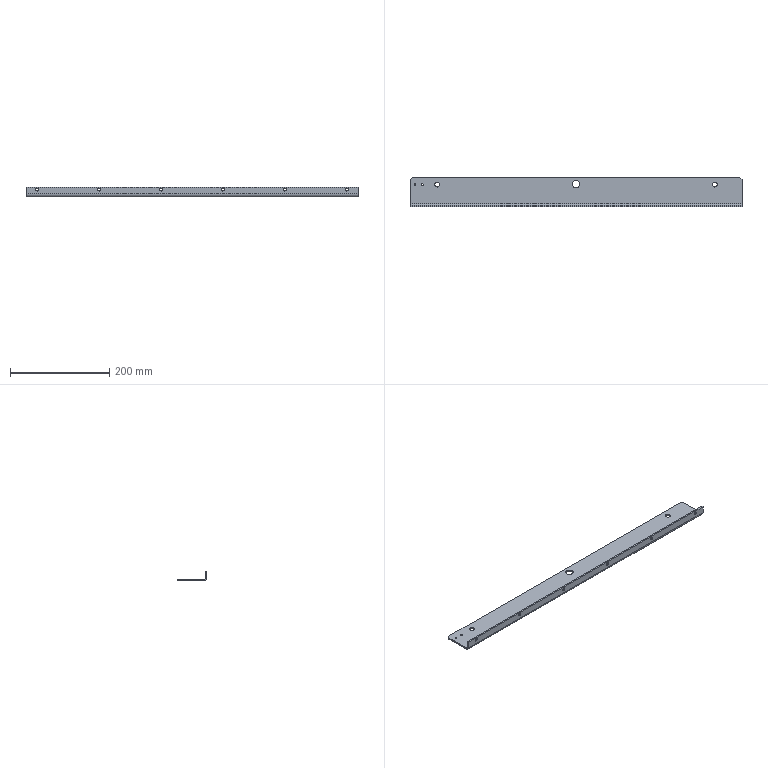Part | NX | features solid 2 | 1 solid | 34 faces | box 670 x 60 x 20 mm | volume 149246 mm3 | cylinder 24 | plane 10 | commonest cylinder face diameters 6 x13 3.459 x4 10 x4 15 x2 12 x1
STEP:
#1=CARTESIAN_POINT('',(-248.27,-1514.473,1300.));
#2=VERTEX_POINT('',#1);
#3=CARTESIAN_POINT('',(-248.27,-1514.473,1303.));
#4=VERTEX_POINT('',#3);
#5=CARTESIAN_POINT('',(-248.27,-1514.473,630.022));
#6=DIRECTION('',(0.,0.,1.));
#7=VECTOR('',#6,1000.);
#8=LINE('',#5,#7);
#9=EDGE_CURVE('',#2,#4,#8,.T.);
#10=ORIENTED_EDGE('',*,*,#9,.F.);
#11=CARTESIAN_POINT('',(-251.73,-1514.473,1300.));
#12=VERTEX_POINT('',#11);
#13=CARTESIAN_POINT('',(-250.,-1514.473,1300.));
#14=DIRECTION('',(0.,0.,-1.));
#15=DIRECTION('',(1.,0.,0.));
#16=AXIS2_PLACEMENT_3D('',#13,#14,#15);
#17=CIRCLE('',#16,1.73);
#18=EDGE_CURVE('',#2,#12,#17,.T.);
#19=ORIENTED_EDGE('',*,*,#18,.T.);
#20=CARTESIAN_POINT('',(-251.73,-1514.473,1303.));
#21=VERTEX_POINT('',#20);
#22=CARTESIAN_POINT('',(-251.73,-1514.473,630.022));
#23=DIRECTION('',(0.,0.,1.));
#24=VECTOR('',#23,1000.);
#25=LINE('',#22,#24);
#26=EDGE_CURVE('',#21,#12,#25,.F.);
#27=ORIENTED_EDGE('',*,*,#26,.F.);
#28=CARTESIAN_POINT('',(-250.,-1514.473,1303.));
#29=DIRECTION('',(0.,0.,1.));
#30=DIRECTION('',(-1.,0.,0.));
#31=AXIS2_PLACEMENT_3D('',#28,#29,#30);
#32=CIRCLE('',#31,1.73);
#33=EDGE_CURVE('',#21,#4,#32,.T.);
#34=ORIENTED_EDGE('',*,*,#33,.T.);
#35=EDGE_LOOP('',(#10,#19,#27,#34));
#36=FACE_BOUND('',#35,.T.);
#37=CARTESIAN_POINT('',(-250.,-1514.473,630.022));
#38=DIRECTION('',(0.,0.,1.));
#39=DIRECTION('',(-1.,0.,0.));
#40=AXIS2_PLACEMENT_3D('',#37,#38,#39);
#41=CYLINDRICAL_SURFACE('',#40,1.73);
#42=ADVANCED_FACE('',(#36),#41,.F.);
#43=CARTESIAN_POINT('',(-233.27,-1514.473,1303.));
#44=VERTEX_POINT('',#43);
#45=CARTESIAN_POINT('',(-233.27,-1514.473,1300.));
#46=VERTEX_POINT('',#45);
#47=CARTESIAN_POINT('',(-233.27,-1514.473,630.022));
#48=DIRECTION('',(0.,0.,1.));
#49=VECTOR('',#48,1000.);
#50=LINE('',#47,#49);
#51=EDGE_CURVE('',#44,#46,#50,.F.);
#52=ORIENTED_EDGE('',*,*,#51,.T.);
#53=CARTESIAN_POINT('',(-236.73,-1514.473,1300.));
#54=VERTEX_POINT('',#53);
#55=CARTESIAN_POINT('',(-235.,-1514.473,1300.));
#56=DIRECTION('',(0.,0.,-1.));
#57=DIRECTION('',(1.,0.,0.));
#58=AXIS2_PLACEMENT_3D('',#55,#56,#57);
#59=CIRCLE('',#58,1.73);
#60=EDGE_CURVE('',#46,#54,#59,.T.);
#61=ORIENTED_EDGE('',*,*,#60,.T.);
#62=CARTESIAN_POINT('',(-236.73,-1514.473,1303.));
#63=VERTEX_POINT('',#62);
#64=CARTESIAN_POINT('',(-236.73,-1514.473,630.022));
#65=DIRECTION('',(0.,0.,1.));
#66=VECTOR('',#65,1000.);
#67=LINE('',#64,#66);
#68=EDGE_CURVE('',#54,#63,#67,.T.);
#69=ORIENTED_EDGE('',*,*,#68,.T.);
#70=CARTESIAN_POINT('',(-235.,-1514.473,1303.));
#71=DIRECTION('',(0.,0.,1.));
#72=DIRECTION('',(-1.,0.,0.));
#73=AXIS2_PLACEMENT_3D('',#70,#71,#72);
#74=CIRCLE('',#73,1.73);
#75=EDGE_CURVE('',#63,#44,#74,.T.);
#76=ORIENTED_EDGE('',*,*,#75,.T.);
#77=EDGE_LOOP('',(#52,#61,#69,#76));
#78=FACE_BOUND('',#77,.T.);
#79=CARTESIAN_POINT('',(-235.,-1514.473,630.022));
#80=DIRECTION('',(0.,0.,1.));
#81=DIRECTION('',(-1.,0.,0.));
#82=AXIS2_PLACEMENT_3D('',#79,#80,#81);
#83=CYLINDRICAL_SURFACE('',#82,1.73);
#84=ADVANCED_FACE('',(#78),#83,.F.);
#85=CARTESIAN_POINT('',(82.5,-1513.723,1300.));
#86=VERTEX_POINT('',#85);
#87=CARTESIAN_POINT('',(82.5,-1513.723,1303.));
#88=VERTEX_POINT('',#87);
#89=CARTESIAN_POINT('',(82.5,-1513.723,630.022));
#90=DIRECTION('',(0.,0.,1.));
#91=VECTOR('',#90,1000.);
#92=LINE('',#89,#91);
#93=EDGE_CURVE('',#86,#88,#92,.T.);
#94=ORIENTED_EDGE('',*,*,#93,.F.);
#95=CARTESIAN_POINT('',(67.5,-1513.723,1300.));
#96=VERTEX_POINT('',#95);
#97=CARTESIAN_POINT('',(75.,-1513.723,1300.));
#98=DIRECTION('',(0.,0.,-1.));
#99=DIRECTION('',(1.,0.,0.));
#100=AXIS2_PLACEMENT_3D('',#97,#98,#99);
#101=CIRCLE('',#100,7.5);
#102=EDGE_CURVE('',#86,#96,#101,.T.);
#103=ORIENTED_EDGE('',*,*,#102,.T.);
#104=CARTESIAN_POINT('',(67.5,-1513.723,1303.));
#105=VERTEX_POINT('',#104);
#106=CARTESIAN_POINT('',(67.5,-1513.723,630.022));
#107=DIRECTION('',(0.,0.,1.));
#108=VECTOR('',#107,1000.);
#109=LINE('',#106,#108);
#110=EDGE_CURVE('',#105,#96,#109,.F.);
#111=ORIENTED_EDGE('',*,*,#110,.F.);
#112=CARTESIAN_POINT('',(75.,-1513.723,1303.));
#113=DIRECTION('',(0.,0.,1.));
#114=DIRECTION('',(1.,0.,0.));
#115=AXIS2_PLACEMENT_3D('',#112,#113,#114);
#116=CIRCLE('',#115,7.5);
#117=EDGE_CURVE('',#105,#88,#116,.T.);
#118=ORIENTED_EDGE('',*,*,#117,.T.);
#119=EDGE_LOOP('',(#94,#103,#111,#118));
#120=FACE_BOUND('',#119,.T.);
#121=CARTESIAN_POINT('',(75.,-1513.723,630.022));
#122=DIRECTION('',(0.,0.,1.));
#123=DIRECTION('',(-1.,0.,0.));
#124=AXIS2_PLACEMENT_3D('',#121,#122,#123);
#125=CYLINDRICAL_SURFACE('',#124,7.5);
#126=ADVANCED_FACE('',(#120),#125,.F.);
#127=CARTESIAN_POINT('',(-255.,-1499.473,1303.));
#128=VERTEX_POINT('',#127);
#129=CARTESIAN_POINT('',(-260.,-1504.473,1303.));
#130=VERTEX_POINT('',#129);
#131=CARTESIAN_POINT('',(-260.,-1504.473,1303.));
#132=DIRECTION('',(-0.7071,-0.7071,0.));
#133=VECTOR('',#132,1000.);
#134=LINE('',#131,#133);
#135=EDGE_CURVE('',#128,#130,#134,.T.);
#136=ORIENTED_EDGE('',*,*,#135,.F.);
#137=CARTESIAN_POINT('',(-255.,-1499.473,1300.));
#138=VERTEX_POINT('',#137);
#139=CARTESIAN_POINT('',(-255.,-1499.473,1300.));
#140=DIRECTION('',(0.,0.,1.));
#141=VECTOR('',#140,1000.);
#142=LINE('',#139,#141);
#143=EDGE_CURVE('',#138,#128,#142,.T.);
#144=ORIENTED_EDGE('',*,*,#143,.F.);
#145=CARTESIAN_POINT('',(-260.,-1504.473,1300.));
#146=VERTEX_POINT('',#145);
#147=CARTESIAN_POINT('',(47.5,-1196.973,1300.));
#148=DIRECTION('',(0.7071,0.7071,0.));
#149=VECTOR('',#148,1000.);
#150=LINE('',#147,#149);
#151=EDGE_CURVE('',#146,#138,#150,.T.);
#152=ORIENTED_EDGE('',*,*,#151,.F.);
#153=CARTESIAN_POINT('',(-260.,-1504.473,1300.));
#154=DIRECTION('',(0.,0.,-1.));
#155=VECTOR('',#154,1000.);
#156=LINE('',#153,#155);
#157=EDGE_CURVE('',#130,#146,#156,.T.);
#158=ORIENTED_EDGE('',*,*,#157,.F.);
#159=EDGE_LOOP('',(#136,#144,#152,#158));
#160=FACE_BOUND('',#159,.T.);
#161=CARTESIAN_POINT('',(-260.,-1504.473,1300.));
#162=DIRECTION('',(0.7071,-0.7071,0.));
#163=DIRECTION('',(0.,0.,-1.));
#164=AXIS2_PLACEMENT_3D('',#161,#162,#163);
#165=PLANE('',#164);
#166=ADVANCED_FACE('',(#160),#165,.F.);
#167=CARTESIAN_POINT('',(410.,-1504.473,1303.));
#168=VERTEX_POINT('',#167);
#169=CARTESIAN_POINT('',(405.,-1499.473,1303.));
#170=VERTEX_POINT('',#169);
#171=CARTESIAN_POINT('',(405.,-1499.473,1303.));
#172=DIRECTION('',(-0.7071,0.7071,0.));
#173=VECTOR('',#172,1000.);
#174=LINE('',#171,#173);
#175=EDGE_CURVE('',#168,#170,#174,.T.);
#176=ORIENTED_EDGE('',*,*,#175,.F.);
#177=CARTESIAN_POINT('',(410.,-1504.473,1300.));
#178=VERTEX_POINT('',#177);
#179=CARTESIAN_POINT('',(410.,-1504.473,1320.));
#180=DIRECTION('',(0.,0.,1.));
#181=VECTOR('',#180,1000.);
#182=LINE('',#179,#181);
#183=EDGE_CURVE('',#178,#168,#182,.T.);
#184=ORIENTED_EDGE('',*,*,#183,.F.);
#185=CARTESIAN_POINT('',(405.,-1499.473,1300.));
#186=VERTEX_POINT('',#185);
#187=CARTESIAN_POINT('',(437.5,-1531.973,1300.));
#188=DIRECTION('',(0.7071,-0.7071,0.));
#189=VECTOR('',#188,1000.);
#190=LINE('',#187,#189);
#191=EDGE_CURVE('',#186,#178,#190,.T.);
#192=ORIENTED_EDGE('',*,*,#191,.F.);
#193=CARTESIAN_POINT('',(405.,-1499.473,1300.));
#194=DIRECTION('',(0.,0.,-1.));
#195=VECTOR('',#194,1000.);
#196=LINE('',#193,#195);
#197=EDGE_CURVE('',#170,#186,#196,.T.);
#198=ORIENTED_EDGE('',*,*,#197,.F.);
#199=EDGE_LOOP('',(#176,#184,#192,#198));
#200=FACE_BOUND('',#199,.T.);
#201=CARTESIAN_POINT('',(405.,-1499.473,1300.));
#202=DIRECTION('',(0.7071,0.7071,0.));
#203=DIRECTION('',(0.,0.,-1.));
#204=AXIS2_PLACEMENT_3D('',#201,#202,#203);
#205=PLANE('',#204);
#206=ADVANCED_FACE('',(#200),#205,.T.);
#207=CARTESIAN_POINT('',(387.5,-1559.473,1318.));
#208=VERTEX_POINT('',#207);
#209=CARTESIAN_POINT('',(387.5,-1556.473,1318.));
#210=VERTEX_POINT('',#209);
#211=CARTESIAN_POINT('',(387.5,-2229.452,1318.));
#212=DIRECTION('',(0.,1.,0.));
#213=VECTOR('',#212,1000.);
#214=LINE('',#211,#213);
#215=EDGE_CURVE('',#208,#210,#214,.T.);
#216=ORIENTED_EDGE('',*,*,#215,.F.);
#217=CARTESIAN_POINT('',(387.5,-1559.473,1312.));
#218=VERTEX_POINT('',#217);
#219=CARTESIAN_POINT('',(387.5,-1559.473,1315.));
#220=DIRECTION('',(0.,-1.,0.));
#221=DIRECTION('',(0.,0.,1.));
#222=AXIS2_PLACEMENT_3D('',#219,#220,#221);
#223=CIRCLE('',#222,3.);
#224=EDGE_CURVE('',#208,#218,#223,.T.);
#225=ORIENTED_EDGE('',*,*,#224,.T.);
#226=CARTESIAN_POINT('',(387.5,-1556.473,1312.));
#227=VERTEX_POINT('',#226);
#228=CARTESIAN_POINT('',(387.5,-2229.452,1312.));
#229=DIRECTION('',(0.,1.,0.));
#230=VECTOR('',#229,1000.);
#231=LINE('',#228,#230);
#232=EDGE_CURVE('',#227,#218,#231,.F.);
#233=ORIENTED_EDGE('',*,*,#232,.F.);
#234=CARTESIAN_POINT('',(387.5,-1556.473,1315.));
#235=DIRECTION('',(0.,1.,0.));
#236=DIRECTION('',(-1.,0.,0.));
#237=AXIS2_PLACEMENT_3D('',#234,#235,#236);
#238=CIRCLE('',#237,3.);
#239=EDGE_CURVE('',#227,#210,#238,.T.);
#240=ORIENTED_EDGE('',*,*,#239,.T.);
#241=EDGE_LOOP('',(#216,#225,#233,#240));
#242=FACE_BOUND('',#241,.T.);
#243=CARTESIAN_POINT('',(387.5,-2229.452,1315.));
#244=DIRECTION('',(0.,1.,0.));
#245=DIRECTION('',(0.,0.,-1.));
#246=AXIS2_PLACEMENT_3D('',#243,#244,#245);
#247=CYLINDRICAL_SURFACE('',#246,3.);
#248=ADVANCED_FACE('',(#242),#247,.F.);
#249=CARTESIAN_POINT('',(-237.5,-1559.473,1318.));
#250=VERTEX_POINT('',#249);
#251=CARTESIAN_POINT('',(-237.5,-1556.473,1318.));
#252=VERTEX_POINT('',#251);
#253=CARTESIAN_POINT('',(-237.5,-2229.452,1318.));
#254=DIRECTION('',(0.,1.,0.));
#255=VECTOR('',#254,1000.);
#256=LINE('',#253,#255);
#257=EDGE_CURVE('',#250,#252,#256,.T.);
#258=ORIENTED_EDGE('',*,*,#257,.F.);
#259=CARTESIAN_POINT('',(-237.5,-1559.473,1312.));
#260=VERTEX_POINT('',#259);
#261=CARTESIAN_POINT('',(-237.5,-1559.473,1315.));
#262=DIRECTION('',(0.,-1.,0.));
#263=DIRECTION('',(0.,0.,1.));
#264=AXIS2_PLACEMENT_3D('',#261,#262,#263);
#265=CIRCLE('',#264,3.);
#266=EDGE_CURVE('',#250,#260,#265,.T.);
#267=ORIENTED_EDGE('',*,*,#266,.T.);
#268=CARTESIAN_POINT('',(-237.5,-1556.473,1312.));
#269=VERTEX_POINT('',#268);
#270=CARTESIAN_POINT('',(-237.5,-2229.452,1312.));
#271=DIRECTION('',(0.,1.,0.));
#272=VECTOR('',#271,1000.);
#273=LINE('',#270,#272);
#274=EDGE_CURVE('',#269,#260,#273,.F.);
#275=ORIENTED_EDGE('',*,*,#274,.F.);
#276=CARTESIAN_POINT('',(-237.5,-1556.473,1315.));
#277=DIRECTION('',(0.,1.,0.));
#278=DIRECTION('',(-1.,0.,0.));
#279=AXIS2_PLACEMENT_3D('',#276,#277,#278);
#280=CIRCLE('',#279,3.);
#281=EDGE_CURVE('',#269,#252,#280,.T.);
#282=ORIENTED_EDGE('',*,*,#281,.T.);
#283=EDGE_LOOP('',(#258,#267,#275,#282));
#284=FACE_BOUND('',#283,.T.);
#285=CARTESIAN_POINT('',(-237.5,-2229.452,1315.));
#286=DIRECTION('',(0.,1.,0.));
#287=DIRECTION('',(0.,0.,-1.));
#288=AXIS2_PLACEMENT_3D('',#285,#286,#287);
#289=CYLINDRICAL_SURFACE('',#288,3.);
#290=ADVANCED_FACE('',(#284),#289,.F.);
#291=CARTESIAN_POINT('',(-112.5,-1556.473,1318.));
#292=VERTEX_POINT('',#291);
#293=CARTESIAN_POINT('',(-112.5,-1559.473,1318.));
#294=VERTEX_POINT('',#293);
#295=CARTESIAN_POINT('',(-112.5,-2229.452,1318.));
#296=DIRECTION('',(0.,1.,0.));
#297=VECTOR('',#296,1000.);
#298=LINE('',#295,#297);
#299=EDGE_CURVE('',#292,#294,#298,.F.);
#300=ORIENTED_EDGE('',*,*,#299,.T.);
#301=CARTESIAN_POINT('',(-112.5,-1559.473,1312.));
#302=VERTEX_POINT('',#301);
#303=CARTESIAN_POINT('',(-112.5,-1559.473,1315.));
#304=DIRECTION('',(0.,-1.,0.));
#305=DIRECTION('',(0.,0.,1.));
#306=AXIS2_PLACEMENT_3D('',#303,#304,#305);
#307=CIRCLE('',#306,3.);
#308=EDGE_CURVE('',#294,#302,#307,.T.);
#309=ORIENTED_EDGE('',*,*,#308,.T.);
#310=CARTESIAN_POINT('',(-112.5,-1556.473,1312.));
#311=VERTEX_POINT('',#310);
#312=CARTESIAN_POINT('',(-112.5,-2229.452,1312.));
#313=DIRECTION('',(0.,1.,0.));
#314=VECTOR('',#313,1000.);
#315=LINE('',#312,#314);
#316=EDGE_CURVE('',#302,#311,#315,.T.);
#317=ORIENTED_EDGE('',*,*,#316,.T.);
#318=CARTESIAN_POINT('',(-112.5,-1556.473,1315.));
#319=DIRECTION('',(0.,1.,0.));
#320=DIRECTION('',(-1.,0.,0.));
#321=AXIS2_PLACEMENT_3D('',#318,#319,#320);
#322=CIRCLE('',#321,3.);
#323=EDGE_CURVE('',#311,#292,#322,.T.);
#324=ORIENTED_EDGE('',*,*,#323,.T.);
#325=EDGE_LOOP('',(#300,#309,#317,#324));
#326=FACE_BOUND('',#325,.T.);
#327=CARTESIAN_POINT('',(-112.5,-2229.452,1315.));
#328=DIRECTION('',(0.,1.,0.));
#329=DIRECTION('',(0.,0.,-1.));
#330=AXIS2_PLACEMENT_3D('',#327,#328,#329);
#331=CYLINDRICAL_SURFACE('',#330,3.);
#332=ADVANCED_FACE('',(#326),#331,.F.);
#333=CARTESIAN_POINT('',(12.5,-1556.473,1318.));
#334=VERTEX_POINT('',#333);
#335=CARTESIAN_POINT('',(12.5,-1559.473,1318.));
#336=VERTEX_POINT('',#335);
#337=CARTESIAN_POINT('',(12.5,-2229.452,1318.));
#338=DIRECTION('',(0.,1.,0.));
#339=VECTOR('',#338,1000.);
#340=LINE('',#337,#339);
#341=EDGE_CURVE('',#334,#336,#340,.F.);
#342=ORIENTED_EDGE('',*,*,#341,.T.);
#343=CARTESIAN_POINT('',(12.5,-1559.473,1312.));
#344=VERTEX_POINT('',#343);
#345=CARTESIAN_POINT('',(12.5,-1559.473,1315.));
#346=DIRECTION('',(0.,-1.,0.));
#347=DIRECTION('',(0.,0.,1.));
#348=AXIS2_PLACEMENT_3D('',#345,#346,#347);
#349=CIRCLE('',#348,3.);
#350=EDGE_CURVE('',#336,#344,#349,.T.);
#351=ORIENTED_EDGE('',*,*,#350,.T.);
#352=CARTESIAN_POINT('',(12.5,-1556.473,1312.));
#353=VERTEX_POINT('',#352);
#354=CARTESIAN_POINT('',(12.5,-2229.452,1312.));
#355=DIRECTION('',(0.,1.,0.));
#356=VECTOR('',#355,1000.);
#357=LINE('',#354,#356);
#358=EDGE_CURVE('',#344,#353,#357,.T.);
#359=ORIENTED_EDGE('',*,*,#358,.T.);
#360=CARTESIAN_POINT('',(12.5,-1556.473,1315.));
#361=DIRECTION('',(0.,1.,0.));
#362=DIRECTION('',(-1.,0.,0.));
#363=AXIS2_PLACEMENT_3D('',#360,#361,#362);
#364=CIRCLE('',#363,3.);
#365=EDGE_CURVE('',#353,#334,#364,.T.);
#366=ORIENTED_EDGE('',*,*,#365,.T.);
#367=EDGE_LOOP('',(#342,#351,#359,#366));
#368=FACE_BOUND('',#367,.T.);
#369=CARTESIAN_POINT('',(12.5,-2229.452,1315.));
#370=DIRECTION('',(0.,1.,0.));
#371=DIRECTION('',(0.,0.,-1.));
#372=AXIS2_PLACEMENT_3D('',#369,#370,#371);
#373=CYLINDRICAL_SURFACE('',#372,3.);
#374=ADVANCED_FACE('',(#368),#373,.F.);
#375=CARTESIAN_POINT('',(137.5,-1559.473,1318.));
#376=VERTEX_POINT('',#375);
#377=CARTESIAN_POINT('',(137.5,-1556.473,1318.));
#378=VERTEX_POINT('',#377);
#379=CARTESIAN_POINT('',(137.5,-2229.452,1318.));
#380=DIRECTION('',(0.,1.,0.));
#381=VECTOR('',#380,1000.);
#382=LINE('',#379,#381);
#383=EDGE_CURVE('',#376,#378,#382,.T.);
#384=ORIENTED_EDGE('',*,*,#383,.F.);
#385=CARTESIAN_POINT('',(137.5,-1559.473,1312.));
#386=VERTEX_POINT('',#385);
#387=CARTESIAN_POINT('',(137.5,-1559.473,1315.));
#388=DIRECTION('',(0.,-1.,0.));
#389=DIRECTION('',(0.,0.,1.));
#390=AXIS2_PLACEMENT_3D('',#387,#388,#389);
#391=CIRCLE('',#390,3.);
#392=EDGE_CURVE('',#376,#386,#391,.T.);
#393=ORIENTED_EDGE('',*,*,#392,.T.);
#394=CARTESIAN_POINT('',(137.5,-1556.473,1312.));
#395=VERTEX_POINT('',#394);
#396=CARTESIAN_POINT('',(137.5,-2229.452,1312.));
#397=DIRECTION('',(0.,1.,0.));
#398=VECTOR('',#397,1000.);
#399=LINE('',#396,#398);
#400=EDGE_CURVE('',#395,#386,#399,.F.);
#401=ORIENTED_EDGE('',*,*,#400,.F.);
#402=CARTESIAN_POINT('',(137.5,-1556.473,1315.));
#403=DIRECTION('',(0.,1.,0.));
#404=DIRECTION('',(-1.,0.,0.));
#405=AXIS2_PLACEMENT_3D('',#402,#403,#404);
#406=CIRCLE('',#405,3.);
#407=EDGE_CURVE('',#395,#378,#406,.T.);
#408=ORIENTED_EDGE('',*,*,#407,.T.);
#409=EDGE_LOOP('',(#384,#393,#401,#408));
#410=FACE_BOUND('',#409,.T.);
#411=CARTESIAN_POINT('',(137.5,-2229.452,1315.));
#412=DIRECTION('',(0.,1.,0.));
#413=DIRECTION('',(0.,0.,-1.));
#414=AXIS2_PLACEMENT_3D('',#411,#412,#413);
#415=CYLINDRICAL_SURFACE('',#414,3.);
#416=ADVANCED_FACE('',(#410),#415,.F.);
#417=CARTESIAN_POINT('',(262.5,-1559.473,1318.));
#418=VERTEX_POINT('',#417);
#419=CARTESIAN_POINT('',(262.5,-1556.473,1318.));
#420=VERTEX_POINT('',#419);
#421=CARTESIAN_POINT('',(262.5,-2229.452,1318.));
#422=DIRECTION('',(0.,1.,0.));
#423=VECTOR('',#422,1000.);
#424=LINE('',#421,#423);
#425=EDGE_CURVE('',#418,#420,#424,.T.);
#426=ORIENTED_EDGE('',*,*,#425,.F.);
#427=CARTESIAN_POINT('',(262.5,-1559.473,1312.));
#428=VERTEX_POINT('',#427);
#429=CARTESIAN_POINT('',(262.5,-1559.473,1315.));
#430=DIRECTION('',(0.,-1.,0.));
#431=DIRECTION('',(0.,0.,1.));
#432=AXIS2_PLACEMENT_3D('',#429,#430,#431);
#433=CIRCLE('',#432,3.);
#434=EDGE_CURVE('',#418,#428,#433,.T.);
#435=ORIENTED_EDGE('',*,*,#434,.T.);
#436=CARTESIAN_POINT('',(262.5,-1556.473,1312.));
#437=VERTEX_POINT('',#436);
#438=CARTESIAN_POINT('',(262.5,-2229.452,1312.));
#439=DIRECTION('',(0.,1.,0.));
#440=VECTOR('',#439,1000.);
#441=LINE('',#438,#440);
#442=EDGE_CURVE('',#437,#428,#441,.F.);
#443=ORIENTED_EDGE('',*,*,#442,.F.);
#444=CARTESIAN_POINT('',(262.5,-1556.473,1315.));
#445=DIRECTION('',(0.,1.,0.));
#446=DIRECTION('',(-1.,0.,0.));
#447=AXIS2_PLACEMENT_3D('',#444,#445,#446);
#448=CIRCLE('',#447,3.);
#449=EDGE_CURVE('',#437,#420,#448,.T.);
#450=ORIENTED_EDGE('',*,*,#449,.T.);
#451=EDGE_LOOP('',(#426,#435,#443,#450));
#452=FACE_BOUND('',#451,.T.);
#453=CARTESIAN_POINT('',(262.5,-2229.452,1315.));
#454=DIRECTION('',(0.,1.,0.));
#455=DIRECTION('',(0.,0.,-1.));
#456=AXIS2_PLACEMENT_3D('',#453,#454,#455);
#457=CYLINDRICAL_SURFACE('',#456,3.);
#458=ADVANCED_FACE('',(#452),#457,.F.);
#459=CARTESIAN_POINT('',(355.,-1519.473,1300.));
#460=VERTEX_POINT('',#459);
#461=CARTESIAN_POINT('',(355.,-1519.473,1303.));
#462=VERTEX_POINT('',#461);
#463=CARTESIAN_POINT('',(355.,-1519.473,630.022));
#464=DIRECTION('',(0.,0.,1.));
#465=VECTOR('',#464,1000.);
#466=LINE('',#463,#465);
#467=EDGE_CURVE('',#460,#462,#466,.T.);
#468=ORIENTED_EDGE('',*,*,#467,.F.);
#469=CARTESIAN_POINT('',(355.,-1509.473,1300.));
#470=VERTEX_POINT('',#469);
#471=CARTESIAN_POINT('',(355.,-1514.473,1300.));
#472=DIRECTION('',(0.,0.,-1.));
#473=DIRECTION('',(1.,0.,0.));
#474=AXIS2_PLACEMENT_3D('',#471,#472,#473);
#475=CIRCLE('',#474,5.);
#476=EDGE_CURVE('',#460,#470,#475,.T.);
#477=ORIENTED_EDGE('',*,*,#476,.T.);
#478=CARTESIAN_POINT('',(355.,-1509.473,1303.));
#479=VERTEX_POINT('',#478);
#480=CARTESIAN_POINT('',(355.,-1509.473,630.022));
#481=DIRECTION('',(0.,0.,1.));
#482=VECTOR('',#481,1000.);
#483=LINE('',#480,#482);
#484=EDGE_CURVE('',#479,#470,#483,.F.);
#485=ORIENTED_EDGE('',*,*,#484,.F.);
#486=CARTESIAN_POINT('',(355.,-1514.473,1303.));
#487=DIRECTION('',(0.,0.,1.));
#488=DIRECTION('',(-1.,0.,0.));
#489=AXIS2_PLACEMENT_3D('',#486,#487,#488);
#490=CIRCLE('',#489,5.);
#491=EDGE_CURVE('',#479,#462,#490,.T.);
#492=ORIENTED_EDGE('',*,*,#491,.T.);
#493=EDGE_LOOP('',(#468,#477,#485,#492));
#494=FACE_BOUND('',#493,.T.);
#495=CARTESIAN_POINT('',(355.,-1514.473,630.022));
#496=DIRECTION('',(0.,0.,1.));
#497=DIRECTION('',(0.,1.,0.));
#498=AXIS2_PLACEMENT_3D('',#495,#496,#497);
#499=CYLINDRICAL_SURFACE('',#498,5.);
#500=ADVANCED_FACE('',(#494),#499,.F.);
#501=CARTESIAN_POINT('',(-205.,-1519.473,1303.));
#502=VERTEX_POINT('',#501);
#503=CARTESIAN_POINT('',(-205.,-1519.473,1300.));
#504=VERTEX_POINT('',#503);
#505=CARTESIAN_POINT('',(-205.,-1519.473,630.022));
#506=DIRECTION('',(0.,0.,1.));
#507=VECTOR('',#506,1000.);
#508=LINE('',#505,#507);
#509=EDGE_CURVE('',#502,#504,#508,.F.);
#510=ORIENTED_EDGE('',*,*,#509,.T.);
#511=CARTESIAN_POINT('',(-205.,-1509.473,1300.));
#512=VERTEX_POINT('',#511);
#513=CARTESIAN_POINT('',(-205.,-1514.473,1300.));
#514=DIRECTION('',(0.,0.,-1.));
#515=DIRECTION('',(1.,0.,0.));
#516=AXIS2_PLACEMENT_3D('',#513,#514,#515);
#517=CIRCLE('',#516,5.);
#518=EDGE_CURVE('',#504,#512,#517,.T.);
#519=ORIENTED_EDGE('',*,*,#518,.T.);
#520=CARTESIAN_POINT('',(-205.,-1509.473,1303.));
#521=VERTEX_POINT('',#520);
#522=CARTESIAN_POINT('',(-205.,-1509.473,630.022));
#523=DIRECTION('',(0.,0.,1.));
#524=VECTOR('',#523,1000.);
#525=LINE('',#522,#524);
#526=EDGE_CURVE('',#512,#521,#525,.T.);
#527=ORIENTED_EDGE('',*,*,#526,.T.);
#528=CARTESIAN_POINT('',(-205.,-1514.473,1303.));
#529=DIRECTION('',(0.,0.,1.));
#530=DIRECTION('',(-1.,0.,0.));
#531=AXIS2_PLACEMENT_3D('',#528,#529,#530);
#532=CIRCLE('',#531,5.);
#533=EDGE_CURVE('',#521,#502,#532,.T.);
#534=ORIENTED_EDGE('',*,*,#533,.T.);
#535=EDGE_LOOP('',(#510,#519,#527,#534));
#536=FACE_BOUND('',#535,.T.);
#537=CARTESIAN_POINT('',(-205.,-1514.473,630.022));
#538=DIRECTION('',(0.,0.,1.));
#539=DIRECTION('',(0.,1.,0.));
#540=AXIS2_PLACEMENT_3D('',#537,#538,#539);
#541=CYLINDRICAL_SURFACE('',#540,5.);
#542=ADVANCED_FACE('',(#536),#541,.F.);
#543=ORIENTED_EDGE('',*,*,#449,.F.);
#544=CARTESIAN_POINT('',(262.5,-1556.473,1315.));
#545=DIRECTION('',(0.,1.,0.));
#546=DIRECTION('',(-1.,0.,0.));
#547=AXIS2_PLACEMENT_3D('',#544,#545,#546);
#548=CIRCLE('',#547,3.);
#549=EDGE_CURVE('',#420,#437,#548,.T.);
#550=ORIENTED_EDGE('',*,*,#549,.F.);
#551=EDGE_LOOP('',(#543,#550));
#552=FACE_BOUND('',#551,.T.);
#553=ORIENTED_EDGE('',*,*,#407,.F.);
#554=CARTESIAN_POINT('',(137.5,-1556.473,1315.));
#555=DIRECTION('',(0.,1.,0.));
#556=DIRECTION('',(-1.,0.,0.));
#557=AXIS2_PLACEMENT_3D('',#554,#555,#556);
#558=CIRCLE('',#557,3.);
#559=EDGE_CURVE('',#378,#395,#558,.T.);
#560=ORIENTED_EDGE('',*,*,#559,.F.);
#561=EDGE_LOOP('',(#553,#560));
#562=FACE_BOUND('',#561,.T.);
#563=ORIENTED_EDGE('',*,*,#365,.F.);
#564=CARTESIAN_POINT('',(12.5,-1556.473,1315.));
#565=DIRECTION('',(0.,1.,0.));
#566=DIRECTION('',(-1.,0.,0.));
#567=AXIS2_PLACEMENT_3D('',#564,#565,#566);
#568=CIRCLE('',#567,3.);
#569=EDGE_CURVE('',#334,#353,#568,.T.);
#570=ORIENTED_EDGE('',*,*,#569,.F.);
#571=EDGE_LOOP('',(#563,#570));
#572=FACE_BOUND('',#571,.T.);
#573=ORIENTED_EDGE('',*,*,#323,.F.);
#574=CARTESIAN_POINT('',(-112.5,-1556.473,1315.));
#575=DIRECTION('',(0.,1.,0.));
#576=DIRECTION('',(-1.,0.,0.));
#577=AXIS2_PLACEMENT_3D('',#574,#575,#576);
#578=CIRCLE('',#577,3.);
#579=EDGE_CURVE('',#292,#311,#578,.T.);
#580=ORIENTED_EDGE('',*,*,#579,.F.);
#581=EDGE_LOOP('',(#573,#580));
#582=FACE_BOUND('',#581,.T.);
#583=ORIENTED_EDGE('',*,*,#281,.F.);
#584=CARTESIAN_POINT('',(-237.5,-1556.473,1315.));
#585=DIRECTION('',(0.,1.,0.));
#586=DIRECTION('',(-1.,0.,0.));
#587=AXIS2_PLACEMENT_3D('',#584,#585,#586);
#588=CIRCLE('',#587,3.);
#589=EDGE_CURVE('',#252,#269,#588,.T.);
#590=ORIENTED_EDGE('',*,*,#589,.F.);
#591=EDGE_LOOP('',(#583,#590));
#592=FACE_BOUND('',#591,.T.);
#593=ORIENTED_EDGE('',*,*,#239,.F.);
#594=CARTESIAN_POINT('',(387.5,-1556.473,1315.));
#595=DIRECTION('',(0.,1.,0.));
#596=DIRECTION('',(-1.,0.,0.));
#597=AXIS2_PLACEMENT_3D('',#594,#595,#596);
#598=CIRCLE('',#597,3.);
#599=EDGE_CURVE('',#210,#227,#598,.T.);
#600=ORIENTED_EDGE('',*,*,#599,.F.);
#601=EDGE_LOOP('',(#593,#600));
#602=FACE_BOUND('',#601,.T.);
#603=CARTESIAN_POINT('',(-260.,-1556.473,1306.));
#604=VERTEX_POINT('',#603);
#605=CARTESIAN_POINT('',(-260.,-1556.473,1320.));
#606=VERTEX_POINT('',#605);
#607=CARTESIAN_POINT('',(-260.,-1556.473,1320.));
#608=DIRECTION('',(0.,0.,1.));
#609=VECTOR('',#608,1000.);
#610=LINE('',#607,#609);
#611=EDGE_CURVE('',#604,#606,#610,.T.);
#612=ORIENTED_EDGE('',*,*,#611,.T.);
#613=CARTESIAN_POINT('',(410.,-1556.473,1320.));
#614=VERTEX_POINT('',#613);
#615=CARTESIAN_POINT('',(410.,-1556.473,1320.));
#616=DIRECTION('',(-1.,0.,0.));
#617=VECTOR('',#616,1000.);
#618=LINE('',#615,#617);
#619=EDGE_CURVE('',#614,#606,#618,.T.);
#620=ORIENTED_EDGE('',*,*,#619,.F.);
#621=CARTESIAN_POINT('',(410.,-1556.473,1306.));
#622=VERTEX_POINT('',#621);
#623=CARTESIAN_POINT('',(410.,-1556.473,1320.));
#624=DIRECTION('',(0.,0.,1.));
#625=VECTOR('',#624,1000.);
#626=LINE('',#623,#625);
#627=EDGE_CURVE('',#622,#614,#626,.T.);
#628=ORIENTED_EDGE('',*,*,#627,.F.);
#629=CARTESIAN_POINT('',(410.,-1556.473,1306.));
#630=DIRECTION('',(-1.,0.,0.));
#631=VECTOR('',#630,1000.);
#632=LINE('',#629,#631);
#633=EDGE_CURVE('',#622,#604,#632,.T.);
#634=ORIENTED_EDGE('',*,*,#633,.T.);
#635=EDGE_LOOP('',(#612,#620,#628,#634));
#636=FACE_BOUND('',#635,.T.);
#637=CARTESIAN_POINT('',(410.,-1556.473,1320.));
#638=DIRECTION('',(0.,-1.,0.));
#639=DIRECTION('',(-1.,0.,0.));
#640=AXIS2_PLACEMENT_3D('',#637,#638,#639);
#641=PLANE('',#640);
#642=ADVANCED_FACE('',(#552,#562,#572,#582,#592,#602,#636),#641,.F.);
#643=CARTESIAN_POINT('',(-260.,-1553.473,1303.));
#644=VERTEX_POINT('',#643);
#645=CARTESIAN_POINT('',(-260.,-1553.473,1306.));
#646=DIRECTION('',(-1.,0.,0.));
#647=DIRECTION('',(0.,0.,-1.));
#648=AXIS2_PLACEMENT_3D('',#645,#646,#647);
#649=CIRCLE('',#648,3.);
#650=EDGE_CURVE('',#644,#604,#649,.T.);
#651=ORIENTED_EDGE('',*,*,#650,.T.);
#652=ORIENTED_EDGE('',*,*,#633,.F.);
#653=CARTESIAN_POINT('',(410.,-1553.473,1303.));
#654=VERTEX_POINT('',#653);
#655=CARTESIAN_POINT('',(410.,-1553.473,1306.));
#656=DIRECTION('',(-1.,0.,0.));
#657=DIRECTION('',(0.,0.,-1.));
#658=AXIS2_PLACEMENT_3D('',#655,#656,#657);
#659=CIRCLE('',#658,3.);
#660=EDGE_CURVE('',#654,#622,#659,.T.);
#661=ORIENTED_EDGE('',*,*,#660,.F.);
#662=CARTESIAN_POINT('',(410.,-1553.473,1303.));
#663=DIRECTION('',(-1.,0.,0.));
#664=VECTOR('',#663,1000.);
#665=LINE('',#662,#664);
#666=EDGE_CURVE('',#654,#644,#665,.T.);
#667=ORIENTED_EDGE('',*,*,#666,.T.);
#668=EDGE_LOOP('',(#651,#652,#661,#667));
#669=FACE_BOUND('',#668,.T.);
#670=CARTESIAN_POINT('',(410.,-1553.473,1306.));
#671=DIRECTION('',(-1.,0.,0.));
#672=DIRECTION('',(0.,0.,-1.));
#673=AXIS2_PLACEMENT_3D('',#670,#671,#672);
#674=CYLINDRICAL_SURFACE('',#673,3.);
#675=ADVANCED_FACE('',(#669),#674,.F.);
#676=ORIENTED_EDGE('',*,*,#533,.F.);
#677=CARTESIAN_POINT('',(-205.,-1514.473,1303.));
#678=DIRECTION('',(0.,0.,1.));
#679=DIRECTION('',(-1.,0.,0.));
#680=AXIS2_PLACEMENT_3D('',#677,#678,#679);
#681=CIRCLE('',#680,5.);
#682=EDGE_CURVE('',#502,#521,#681,.T.);
#683=ORIENTED_EDGE('',*,*,#682,.F.);
#684=EDGE_LOOP('',(#676,#683));
#685=FACE_BOUND('',#684,.T.);
#686=ORIENTED_EDGE('',*,*,#491,.F.);
#687=CARTESIAN_POINT('',(355.,-1514.473,1303.));
#688=DIRECTION('',(0.,0.,1.));
#689=DIRECTION('',(-1.,0.,0.));
#690=AXIS2_PLACEMENT_3D('',#687,#688,#689);
#691=CIRCLE('',#690,5.);
#692=EDGE_CURVE('',#462,#479,#691,.T.);
#693=ORIENTED_EDGE('',*,*,#692,.F.);
#694=EDGE_LOOP('',(#686,#693));
#695=FACE_BOUND('',#694,.T.);
#696=ORIENTED_EDGE('',*,*,#117,.F.);
#697=CARTESIAN_POINT('',(75.,-1513.723,1303.));
#698=DIRECTION('',(0.,0.,1.));
#699=DIRECTION('',(1.,0.,0.));
#700=AXIS2_PLACEMENT_3D('',#697,#698,#699);
#701=CIRCLE('',#700,7.5);
#702=EDGE_CURVE('',#88,#105,#701,.T.);
#703=ORIENTED_EDGE('',*,*,#702,.F.);
#704=EDGE_LOOP('',(#696,#703));
#705=FACE_BOUND('',#704,.T.);
#706=ORIENTED_EDGE('',*,*,#75,.F.);
#707=CARTESIAN_POINT('',(-235.,-1514.473,1303.));
#708=DIRECTION('',(0.,0.,1.));
#709=DIRECTION('',(-1.,0.,0.));
#710=AXIS2_PLACEMENT_3D('',#707,#708,#709);
#711=CIRCLE('',#710,1.73);
#712=EDGE_CURVE('',#44,#63,#711,.T.);
#713=ORIENTED_EDGE('',*,*,#712,.F.);
#714=EDGE_LOOP('',(#706,#713));
#715=FACE_BOUND('',#714,.T.);
#716=ORIENTED_EDGE('',*,*,#33,.F.);
#717=CARTESIAN_POINT('',(-250.,-1514.473,1303.));
#718=DIRECTION('',(0.,0.,1.));
#719=DIRECTION('',(-1.,0.,0.));
#720=AXIS2_PLACEMENT_3D('',#717,#718,#719);
#721=CIRCLE('',#720,1.73);
#722=EDGE_CURVE('',#4,#21,#721,.T.);
#723=ORIENTED_EDGE('',*,*,#722,.F.);
#724=EDGE_LOOP('',(#716,#723));
#725=FACE_BOUND('',#724,.T.);
#726=CARTESIAN_POINT('',(410.,-1559.473,1303.));
#727=DIRECTION('',(0.,-1.,0.));
#728=VECTOR('',#727,1000.);
#729=LINE('',#726,#728);
#730=EDGE_CURVE('',#168,#654,#729,.T.);
#731=ORIENTED_EDGE('',*,*,#730,.F.);
#732=ORIENTED_EDGE('',*,*,#175,.T.);
#733=CARTESIAN_POINT('',(410.,-1499.473,1303.));
#734=DIRECTION('',(-1.,0.,0.));
#735=VECTOR('',#734,1000.);
#736=LINE('',#733,#735);
#737=EDGE_CURVE('',#170,#128,#736,.T.);
#738=ORIENTED_EDGE('',*,*,#737,.T.);
#739=ORIENTED_EDGE('',*,*,#135,.T.);
#740=CARTESIAN_POINT('',(-260.,-1559.473,1303.));
#741=DIRECTION('',(0.,-1.,0.));
#742=VECTOR('',#741,1000.);
#743=LINE('',#740,#742);
#744=EDGE_CURVE('',#130,#644,#743,.T.);
#745=ORIENTED_EDGE('',*,*,#744,.T.);
#746=ORIENTED_EDGE('',*,*,#666,.F.);
#747=EDGE_LOOP('',(#731,#732,#738,#739,#745,#746));
#748=FACE_BOUND('',#747,.T.);
#749=CARTESIAN_POINT('',(410.,-1559.473,1303.));
#750=DIRECTION('',(0.,0.,-1.));
#751=DIRECTION('',(0.,-1.,0.));
#752=AXIS2_PLACEMENT_3D('',#749,#750,#751);
#753=PLANE('',#752);
#754=ADVANCED_FACE('',(#685,#695,#705,#715,#725,#748),#753,.F.);
#755=CARTESIAN_POINT('',(262.5,-1559.473,1315.));
#756=DIRECTION('',(0.,-1.,0.));
#757=DIRECTION('',(0.,0.,1.));
#758=AXIS2_PLACEMENT_3D('',#755,#756,#757);
#759=CIRCLE('',#758,3.);
#760=EDGE_CURVE('',#428,#418,#759,.T.);
#761=ORIENTED_EDGE('',*,*,#760,.F.);
#762=ORIENTED_EDGE('',*,*,#434,.F.);
#763=EDGE_LOOP('',(#761,#762));
#764=FACE_BOUND('',#763,.T.);
#765=CARTESIAN_POINT('',(137.5,-1559.473,1315.));
#766=DIRECTION('',(0.,-1.,0.));
#767=DIRECTION('',(0.,0.,1.));
#768=AXIS2_PLACEMENT_3D('',#765,#766,#767);
#769=CIRCLE('',#768,3.);
#770=EDGE_CURVE('',#386,#376,#769,.T.);
#771=ORIENTED_EDGE('',*,*,#770,.F.);
#772=ORIENTED_EDGE('',*,*,#392,.F.);
#773=EDGE_LOOP('',(#771,#772));
#774=FACE_BOUND('',#773,.T.);
#775=CARTESIAN_POINT('',(12.5,-1559.473,1315.));
#776=DIRECTION('',(0.,-1.,0.));
#777=DIRECTION('',(0.,0.,1.));
#778=AXIS2_PLACEMENT_3D('',#775,#776,#777);
#779=CIRCLE('',#778,3.);
#780=EDGE_CURVE('',#344,#336,#779,.T.);
#781=ORIENTED_EDGE('',*,*,#780,.F.);
#782=ORIENTED_EDGE('',*,*,#350,.F.);
#783=EDGE_LOOP('',(#781,#782));
#784=FACE_BOUND('',#783,.T.);
#785=CARTESIAN_POINT('',(-112.5,-1559.473,1315.));
#786=DIRECTION('',(0.,-1.,0.));
#787=DIRECTION('',(0.,0.,1.));
#788=AXIS2_PLACEMENT_3D('',#785,#786,#787);
#789=CIRCLE('',#788,3.);
#790=EDGE_CURVE('',#302,#294,#789,.T.);
#791=ORIENTED_EDGE('',*,*,#790,.F.);
#792=ORIENTED_EDGE('',*,*,#308,.F.);
#793=EDGE_LOOP('',(#791,#792));
#794=FACE_BOUND('',#793,.T.);
#795=CARTESIAN_POINT('',(-237.5,-1559.473,1315.));
#796=DIRECTION('',(0.,-1.,0.));
#797=DIRECTION('',(0.,0.,1.));
#798=AXIS2_PLACEMENT_3D('',#795,#796,#797);
#799=CIRCLE('',#798,3.);
#800=EDGE_CURVE('',#260,#250,#799,.T.);
#801=ORIENTED_EDGE('',*,*,#800,.F.);
#802=ORIENTED_EDGE('',*,*,#266,.F.);
#803=EDGE_LOOP('',(#801,#802));
#804=FACE_BOUND('',#803,.T.);
#805=CARTESIAN_POINT('',(387.5,-1559.473,1315.));
#806=DIRECTION('',(0.,-1.,0.));
#807=DIRECTION('',(0.,0.,1.));
#808=AXIS2_PLACEMENT_3D('',#805,#806,#807);
#809=CIRCLE('',#808,3.);
#810=EDGE_CURVE('',#218,#208,#809,.T.);
#811=ORIENTED_EDGE('',*,*,#810,.F.);
#812=ORIENTED_EDGE('',*,*,#224,.F.);
#813=EDGE_LOOP('',(#811,#812));
#814=FACE_BOUND('',#813,.T.);
#815=CARTESIAN_POINT('',(-260.,-1559.473,1306.));
#816=VERTEX_POINT('',#815);
#817=CARTESIAN_POINT('',(-260.,-1559.473,1320.));
#818=VERTEX_POINT('',#817);
#819=CARTESIAN_POINT('',(-260.,-1559.473,1320.));
#820=DIRECTION('',(0.,0.,1.));
#821=VECTOR('',#820,1000.);
#822=LINE('',#819,#821);
#823=EDGE_CURVE('',#816,#818,#822,.T.);
#824=ORIENTED_EDGE('',*,*,#823,.F.);
#825=CARTESIAN_POINT('',(410.,-1559.473,1306.));
#826=VERTEX_POINT('',#825);
#827=CARTESIAN_POINT('',(410.,-1559.473,1306.));
#828=DIRECTION('',(-1.,0.,0.));
#829=VECTOR('',#828,1000.);
#830=LINE('',#827,#829);
#831=EDGE_CURVE('',#826,#816,#830,.T.);
#832=ORIENTED_EDGE('',*,*,#831,.F.);
#833=CARTESIAN_POINT('',(410.,-1559.473,1320.));
#834=VERTEX_POINT('',#833);
#835=CARTESIAN_POINT('',(410.,-1559.473,1320.));
#836=DIRECTION('',(0.,0.,1.));
#837=VECTOR('',#836,1000.);
#838=LINE('',#835,#837);
#839=EDGE_CURVE('',#826,#834,#838,.T.);
#840=ORIENTED_EDGE('',*,*,#839,.T.);
#841=CARTESIAN_POINT('',(410.,-1559.473,1320.));
#842=DIRECTION('',(-1.,0.,0.));
#843=VECTOR('',#842,1000.);
#844=LINE('',#841,#843);
#845=EDGE_CURVE('',#834,#818,#844,.T.);
#846=ORIENTED_EDGE('',*,*,#845,.T.);
#847=EDGE_LOOP('',(#824,#832,#840,#846));
#848=FACE_BOUND('',#847,.T.);
#849=CARTESIAN_POINT('',(410.,-1559.473,1320.));
#850=DIRECTION('',(0.,-1.,0.));
#851=DIRECTION('',(-1.,0.,0.));
#852=AXIS2_PLACEMENT_3D('',#849,#850,#851);
#853=PLANE('',#852);
#854=ADVANCED_FACE('',(#764,#774,#784,#794,#804,#814,#848),#853,.T.);
#855=CARTESIAN_POINT('',(-260.,-1553.473,1300.));
#856=VERTEX_POINT('',#855);
#857=CARTESIAN_POINT('',(-260.,-1553.473,1306.));
#858=DIRECTION('',(-1.,0.,0.));
#859=DIRECTION('',(0.,1.,0.));
#860=AXIS2_PLACEMENT_3D('',#857,#858,#859);
#861=CIRCLE('',#860,6.);
#862=EDGE_CURVE('',#856,#816,#861,.T.);
#863=ORIENTED_EDGE('',*,*,#862,.F.);
#864=CARTESIAN_POINT('',(410.,-1553.473,1300.));
#865=VERTEX_POINT('',#864);
#866=CARTESIAN_POINT('',(410.,-1553.473,1300.));
#867=DIRECTION('',(-1.,0.,0.));
#868=VECTOR('',#867,1000.);
#869=LINE('',#866,#868);
#870=EDGE_CURVE('',#865,#856,#869,.T.);
#871=ORIENTED_EDGE('',*,*,#870,.F.);
#872=CARTESIAN_POINT('',(410.,-1553.473,1306.));
#873=DIRECTION('',(-1.,0.,0.));
#874=DIRECTION('',(0.,1.,0.));
#875=AXIS2_PLACEMENT_3D('',#872,#873,#874);
#876=CIRCLE('',#875,6.);
#877=EDGE_CURVE('',#865,#826,#876,.T.);
#878=ORIENTED_EDGE('',*,*,#877,.T.);
#879=ORIENTED_EDGE('',*,*,#831,.T.);
#880=EDGE_LOOP('',(#863,#871,#878,#879));
#881=FACE_BOUND('',#880,.T.);
#882=CARTESIAN_POINT('',(410.,-1553.473,1306.));
#883=DIRECTION('',(-1.,0.,0.));
#884=DIRECTION('',(0.,0.,-1.));
#885=AXIS2_PLACEMENT_3D('',#882,#883,#884);
#886=CYLINDRICAL_SURFACE('',#885,6.);
#887=ADVANCED_FACE('',(#881),#886,.T.);
#888=CARTESIAN_POINT('',(-205.,-1514.473,1300.));
#889=DIRECTION('',(0.,0.,-1.));
#890=DIRECTION('',(1.,0.,0.));
#891=AXIS2_PLACEMENT_3D('',#888,#889,#890);
#892=CIRCLE('',#891,5.);
#893=EDGE_CURVE('',#512,#504,#892,.T.);
#894=ORIENTED_EDGE('',*,*,#893,.F.);
#895=ORIENTED_EDGE('',*,*,#518,.F.);
#896=EDGE_LOOP('',(#894,#895));
#897=FACE_BOUND('',#896,.T.);
#898=CARTESIAN_POINT('',(355.,-1514.473,1300.));
#899=DIRECTION('',(0.,0.,-1.));
#900=DIRECTION('',(1.,0.,0.));
#901=AXIS2_PLACEMENT_3D('',#898,#899,#900);
#902=CIRCLE('',#901,5.);
#903=EDGE_CURVE('',#470,#460,#902,.T.);
#904=ORIENTED_EDGE('',*,*,#903,.F.);
#905=ORIENTED_EDGE('',*,*,#476,.F.);
#906=EDGE_LOOP('',(#904,#905));
#907=FACE_BOUND('',#906,.T.);
#908=CARTESIAN_POINT('',(75.,-1513.723,1300.));
#909=DIRECTION('',(0.,0.,-1.));
#910=DIRECTION('',(1.,0.,0.));
#911=AXIS2_PLACEMENT_3D('',#908,#909,#910);
#912=CIRCLE('',#911,7.5);
#913=EDGE_CURVE('',#96,#86,#912,.T.);
#914=ORIENTED_EDGE('',*,*,#913,.F.);
#915=ORIENTED_EDGE('',*,*,#102,.F.);
#916=EDGE_LOOP('',(#914,#915));
#917=FACE_BOUND('',#916,.T.);
#918=CARTESIAN_POINT('',(-235.,-1514.473,1300.));
#919=DIRECTION('',(0.,0.,-1.));
#920=DIRECTION('',(1.,0.,0.));
#921=AXIS2_PLACEMENT_3D('',#918,#919,#920);
#922=CIRCLE('',#921,1.73);
#923=EDGE_CURVE('',#54,#46,#922,.T.);
#924=ORIENTED_EDGE('',*,*,#923,.F.);
#925=ORIENTED_EDGE('',*,*,#60,.F.);
#926=EDGE_LOOP('',(#924,#925));
#927=FACE_BOUND('',#926,.T.);
#928=CARTESIAN_POINT('',(-250.,-1514.473,1300.));
#929=DIRECTION('',(0.,0.,-1.));
#930=DIRECTION('',(1.,0.,0.));
#931=AXIS2_PLACEMENT_3D('',#928,#929,#930);
#932=CIRCLE('',#931,1.73);
#933=EDGE_CURVE('',#12,#2,#932,.T.);
#934=ORIENTED_EDGE('',*,*,#933,.F.);
#935=ORIENTED_EDGE('',*,*,#18,.F.);
#936=EDGE_LOOP('',(#934,#935));
#937=FACE_BOUND('',#936,.T.);
#938=CARTESIAN_POINT('',(410.,-1499.473,1300.));
#939=DIRECTION('',(-1.,0.,0.));
#940=VECTOR('',#939,1000.);
#941=LINE('',#938,#940);
#942=EDGE_CURVE('',#186,#138,#941,.T.);
#943=ORIENTED_EDGE('',*,*,#942,.F.);
#944=ORIENTED_EDGE('',*,*,#191,.T.);
#945=CARTESIAN_POINT('',(410.,-1559.473,1300.));
#946=DIRECTION('',(0.,-1.,0.));
#947=VECTOR('',#946,1000.);
#948=LINE('',#945,#947);
#949=EDGE_CURVE('',#178,#865,#948,.T.);
#950=ORIENTED_EDGE('',*,*,#949,.T.);
#951=ORIENTED_EDGE('',*,*,#870,.T.);
#952=CARTESIAN_POINT('',(-260.,-1559.473,1300.));
#953=DIRECTION('',(0.,-1.,0.));
#954=VECTOR('',#953,1000.);
#955=LINE('',#952,#954);
#956=EDGE_CURVE('',#146,#856,#955,.T.);
#957=ORIENTED_EDGE('',*,*,#956,.F.);
#958=ORIENTED_EDGE('',*,*,#151,.T.);
#959=EDGE_LOOP('',(#943,#944,#950,#951,#957,#958));
#960=FACE_BOUND('',#959,.T.);
#961=CARTESIAN_POINT('',(410.,-1559.473,1300.));
#962=DIRECTION('',(0.,0.,-1.));
#963=DIRECTION('',(0.,-1.,0.));
#964=AXIS2_PLACEMENT_3D('',#961,#962,#963);
#965=PLANE('',#964);
#966=ADVANCED_FACE('',(#897,#907,#917,#927,#937,#960),#965,.T.);
#967=ORIENTED_EDGE('',*,*,#737,.F.);
#968=ORIENTED_EDGE('',*,*,#197,.T.);
#969=ORIENTED_EDGE('',*,*,#942,.T.);
#970=ORIENTED_EDGE('',*,*,#143,.T.);
#971=EDGE_LOOP('',(#967,#968,#969,#970));
#972=FACE_BOUND('',#971,.T.);
#973=CARTESIAN_POINT('',(410.,-1499.473,1300.));
#974=DIRECTION('',(0.,-1.,0.));
#975=DIRECTION('',(-1.,0.,0.));
#976=AXIS2_PLACEMENT_3D('',#973,#974,#975);
#977=PLANE('',#976);
#978=ADVANCED_FACE('',(#972),#977,.F.);
#979=ORIENTED_EDGE('',*,*,#744,.F.);
#980=ORIENTED_EDGE('',*,*,#157,.T.);
#981=ORIENTED_EDGE('',*,*,#956,.T.);
#982=ORIENTED_EDGE('',*,*,#862,.T.);
#983=ORIENTED_EDGE('',*,*,#823,.T.);
#984=CARTESIAN_POINT('',(-260.,-1559.473,1320.));
#985=DIRECTION('',(0.,-1.,0.));
#986=VECTOR('',#985,1000.);
#987=LINE('',#984,#986);
#988=EDGE_CURVE('',#606,#818,#987,.T.);
#989=ORIENTED_EDGE('',*,*,#988,.F.);
#990=ORIENTED_EDGE('',*,*,#611,.F.);
#991=ORIENTED_EDGE('',*,*,#650,.F.);
#992=EDGE_LOOP('',(#979,#980,#981,#982,#983,#989,#990,#991));
#993=FACE_BOUND('',#992,.T.);
#994=CARTESIAN_POINT('',(-260.,-1559.473,1300.));
#995=DIRECTION('',(1.,0.,0.));
#996=DIRECTION('',(0.,0.,-1.));
#997=AXIS2_PLACEMENT_3D('',#994,#995,#996);
#998=PLANE('',#997);
#999=ADVANCED_FACE('',(#993),#998,.F.);
#1000=CARTESIAN_POINT('',(410.,-1559.473,1320.));
#1001=DIRECTION('',(0.,-1.,0.));
#1002=VECTOR('',#1001,1000.);
#1003=LINE('',#1000,#1002);
#1004=EDGE_CURVE('',#614,#834,#1003,.T.);
#1005=ORIENTED_EDGE('',*,*,#1004,.F.);
#1006=ORIENTED_EDGE('',*,*,#619,.T.);
#1007=ORIENTED_EDGE('',*,*,#988,.T.);
#1008=ORIENTED_EDGE('',*,*,#845,.F.);
#1009=EDGE_LOOP('',(#1005,#1006,#1007,#1008));
#1010=FACE_BOUND('',#1009,.T.);
#1011=CARTESIAN_POINT('',(410.,-1559.473,1320.));
#1012=DIRECTION('',(0.,0.,1.));
#1013=DIRECTION('',(0.,-1.,0.));
#1014=AXIS2_PLACEMENT_3D('',#1011,#1012,#1013);
#1015=PLANE('',#1014);
#1016=ADVANCED_FACE('',(#1010),#1015,.T.);
#1017=ORIENTED_EDGE('',*,*,#949,.F.);
#1018=ORIENTED_EDGE('',*,*,#183,.T.);
#1019=ORIENTED_EDGE('',*,*,#730,.T.);
#1020=ORIENTED_EDGE('',*,*,#660,.T.);
#1021=ORIENTED_EDGE('',*,*,#627,.T.);
#1022=ORIENTED_EDGE('',*,*,#1004,.T.);
#1023=ORIENTED_EDGE('',*,*,#839,.F.);
#1024=ORIENTED_EDGE('',*,*,#877,.F.);
#1025=EDGE_LOOP('',(#1017,#1018,#1019,#1020,#1021,#1022,#1023,#1024));
#1026=FACE_BOUND('',#1025,.T.);
#1027=CARTESIAN_POINT('',(410.,-1559.473,1320.));
#1028=DIRECTION('',(1.,0.,0.));
#1029=DIRECTION('',(0.,0.,-1.));
#1030=AXIS2_PLACEMENT_3D('',#1027,#1028,#1029);
#1031=PLANE('',#1030);
#1032=ADVANCED_FACE('',(#1026),#1031,.T.);
#1033=ORIENTED_EDGE('',*,*,#893,.T.);
#1034=ORIENTED_EDGE('',*,*,#509,.F.);
#1035=ORIENTED_EDGE('',*,*,#682,.T.);
#1036=ORIENTED_EDGE('',*,*,#526,.F.);
#1037=EDGE_LOOP('',(#1033,#1034,#1035,#1036));
#1038=FACE_BOUND('',#1037,.T.);
#1039=CARTESIAN_POINT('',(-205.,-1514.473,630.022));
#1040=DIRECTION('',(0.,0.,1.));
#1041=DIRECTION('',(0.,1.,0.));
#1042=AXIS2_PLACEMENT_3D('',#1039,#1040,#1041);
#1043=CYLINDRICAL_SURFACE('',#1042,5.);
#1044=ADVANCED_FACE('',(#1038),#1043,.F.);
#1045=ORIENTED_EDGE('',*,*,#903,.T.);
#1046=ORIENTED_EDGE('',*,*,#467,.T.);
#1047=ORIENTED_EDGE('',*,*,#692,.T.);
#1048=ORIENTED_EDGE('',*,*,#484,.T.);
#1049=EDGE_LOOP('',(#1045,#1046,#1047,#1048));
#1050=FACE_BOUND('',#1049,.T.);
#1051=CARTESIAN_POINT('',(355.,-1514.473,630.022));
#1052=DIRECTION('',(0.,0.,1.));
#1053=DIRECTION('',(0.,1.,0.));
#1054=AXIS2_PLACEMENT_3D('',#1051,#1052,#1053);
#1055=CYLINDRICAL_SURFACE('',#1054,5.);
#1056=ADVANCED_FACE('',(#1050),#1055,.F.);
#1057=ORIENTED_EDGE('',*,*,#760,.T.);
#1058=ORIENTED_EDGE('',*,*,#425,.T.);
#1059=ORIENTED_EDGE('',*,*,#549,.T.);
#1060=ORIENTED_EDGE('',*,*,#442,.T.);
#1061=EDGE_LOOP('',(#1057,#1058,#1059,#1060));
#1062=FACE_BOUND('',#1061,.T.);
#1063=CARTESIAN_POINT('',(262.5,-2229.452,1315.));
#1064=DIRECTION('',(0.,1.,0.));
#1065=DIRECTION('',(0.,0.,-1.));
#1066=AXIS2_PLACEMENT_3D('',#1063,#1064,#1065);
#1067=CYLINDRICAL_SURFACE('',#1066,3.);
#1068=ADVANCED_FACE('',(#1062),#1067,.F.);
#1069=ORIENTED_EDGE('',*,*,#770,.T.);
#1070=ORIENTED_EDGE('',*,*,#383,.T.);
#1071=ORIENTED_EDGE('',*,*,#559,.T.);
#1072=ORIENTED_EDGE('',*,*,#400,.T.);
#1073=EDGE_LOOP('',(#1069,#1070,#1071,#1072));
#1074=FACE_BOUND('',#1073,.T.);
#1075=CARTESIAN_POINT('',(137.5,-2229.452,1315.));
#1076=DIRECTION('',(0.,1.,0.));
#1077=DIRECTION('',(0.,0.,-1.));
#1078=AXIS2_PLACEMENT_3D('',#1075,#1076,#1077);
#1079=CYLINDRICAL_SURFACE('',#1078,3.);
#1080=ADVANCED_FACE('',(#1074),#1079,.F.);
#1081=ORIENTED_EDGE('',*,*,#780,.T.);
#1082=ORIENTED_EDGE('',*,*,#341,.F.);
#1083=ORIENTED_EDGE('',*,*,#569,.T.);
#1084=ORIENTED_EDGE('',*,*,#358,.F.);
#1085=EDGE_LOOP('',(#1081,#1082,#1083,#1084));
#1086=FACE_BOUND('',#1085,.T.);
#1087=CARTESIAN_POINT('',(12.5,-2229.452,1315.));
#1088=DIRECTION('',(0.,1.,0.));
#1089=DIRECTION('',(0.,0.,-1.));
#1090=AXIS2_PLACEMENT_3D('',#1087,#1088,#1089);
#1091=CYLINDRICAL_SURFACE('',#1090,3.);
#1092=ADVANCED_FACE('',(#1086),#1091,.F.);
#1093=ORIENTED_EDGE('',*,*,#790,.T.);
#1094=ORIENTED_EDGE('',*,*,#299,.F.);
#1095=ORIENTED_EDGE('',*,*,#579,.T.);
#1096=ORIENTED_EDGE('',*,*,#316,.F.);
#1097=EDGE_LOOP('',(#1093,#1094,#1095,#1096));
#1098=FACE_BOUND('',#1097,.T.);
#1099=CARTESIAN_POINT('',(-112.5,-2229.452,1315.));
#1100=DIRECTION('',(0.,1.,0.));
#1101=DIRECTION('',(0.,0.,-1.));
#1102=AXIS2_PLACEMENT_3D('',#1099,#1100,#1101);
#1103=CYLINDRICAL_SURFACE('',#1102,3.);
#1104=ADVANCED_FACE('',(#1098),#1103,.F.);
#1105=ORIENTED_EDGE('',*,*,#800,.T.);
#1106=ORIENTED_EDGE('',*,*,#257,.T.);
#1107=ORIENTED_EDGE('',*,*,#589,.T.);
#1108=ORIENTED_EDGE('',*,*,#274,.T.);
#1109=EDGE_LOOP('',(#1105,#1106,#1107,#1108));
#1110=FACE_BOUND('',#1109,.T.);
#1111=CARTESIAN_POINT('',(-237.5,-2229.452,1315.));
#1112=DIRECTION('',(0.,1.,0.));
#1113=DIRECTION('',(0.,0.,-1.));
#1114=AXIS2_PLACEMENT_3D('',#1111,#1112,#1113);
#1115=CYLINDRICAL_SURFACE('',#1114,3.);
#1116=ADVANCED_FACE('',(#1110),#1115,.F.);
#1117=ORIENTED_EDGE('',*,*,#810,.T.);
#1118=ORIENTED_EDGE('',*,*,#215,.T.);
#1119=ORIENTED_EDGE('',*,*,#599,.T.);
#1120=ORIENTED_EDGE('',*,*,#232,.T.);
#1121=EDGE_LOOP('',(#1117,#1118,#1119,#1120));
#1122=FACE_BOUND('',#1121,.T.);
#1123=CARTESIAN_POINT('',(387.5,-2229.452,1315.));
#1124=DIRECTION('',(0.,1.,0.));
#1125=DIRECTION('',(0.,0.,-1.));
#1126=AXIS2_PLACEMENT_3D('',#1123,#1124,#1125);
#1127=CYLINDRICAL_SURFACE('',#1126,3.);
#1128=ADVANCED_FACE('',(#1122),#1127,.F.);
#1129=ORIENTED_EDGE('',*,*,#913,.T.);
#1130=ORIENTED_EDGE('',*,*,#93,.T.);
#1131=ORIENTED_EDGE('',*,*,#702,.T.);
#1132=ORIENTED_EDGE('',*,*,#110,.T.);
#1133=EDGE_LOOP('',(#1129,#1130,#1131,#1132));
#1134=FACE_BOUND('',#1133,.T.);
#1135=CARTESIAN_POINT('',(75.,-1513.723,630.022));
#1136=DIRECTION('',(0.,0.,1.));
#1137=DIRECTION('',(-1.,0.,0.));
#1138=AXIS2_PLACEMENT_3D('',#1135,#1136,#1137);
#1139=CYLINDRICAL_SURFACE('',#1138,7.5);
#1140=ADVANCED_FACE('',(#1134),#1139,.F.);
#1141=ORIENTED_EDGE('',*,*,#923,.T.);
#1142=ORIENTED_EDGE('',*,*,#51,.F.);
#1143=ORIENTED_EDGE('',*,*,#712,.T.);
#1144=ORIENTED_EDGE('',*,*,#68,.F.);
#1145=EDGE_LOOP('',(#1141,#1142,#1143,#1144));
#1146=FACE_BOUND('',#1145,.T.);
#1147=CARTESIAN_POINT('',(-235.,-1514.473,630.022));
#1148=DIRECTION('',(0.,0.,1.));
#1149=DIRECTION('',(-1.,0.,0.));
#1150=AXIS2_PLACEMENT_3D('',#1147,#1148,#1149);
#1151=CYLINDRICAL_SURFACE('',#1150,1.73);
#1152=ADVANCED_FACE('',(#1146),#1151,.F.);
#1153=ORIENTED_EDGE('',*,*,#933,.T.);
#1154=ORIENTED_EDGE('',*,*,#9,.T.);
#1155=ORIENTED_EDGE('',*,*,#722,.T.);
#1156=ORIENTED_EDGE('',*,*,#26,.T.);
#1157=EDGE_LOOP('',(#1153,#1154,#1155,#1156));
#1158=FACE_BOUND('',#1157,.T.);
#1159=CARTESIAN_POINT('',(-250.,-1514.473,630.022));
#1160=DIRECTION('',(0.,0.,1.));
#1161=DIRECTION('',(-1.,0.,0.));
#1162=AXIS2_PLACEMENT_3D('',#1159,#1160,#1161);
#1163=CYLINDRICAL_SURFACE('',#1162,1.73);
#1164=ADVANCED_FACE('',(#1158),#1163,.F.);
#1165=CLOSED_SHELL('',(#42,#84,#126,#166,#206,#248,#290,#332,#374,#416,#458,#500,#542,#642,#675,#754,#854,#887,#966,#978,#999,#1016,#1032,#1044,#1056,#1068,#1080,#1092,#1104,#1116,#1128,#1140,#1152,#1164));
#1166=MANIFOLD_SOLID_BREP('',#1165);
#1167=(LENGTH_UNIT()NAMED_UNIT(*)SI_UNIT(.MILLI.,.METRE.));
#1168=UNCERTAINTY_MEASURE_WITH_UNIT(LENGTH_MEASURE(0.00001),#1167,'','');
#1169=(NAMED_UNIT(*)PLANE_ANGLE_UNIT()SI_UNIT($,.RADIAN.));
#1170=(NAMED_UNIT(*)SI_UNIT($,.STERADIAN.)SOLID_ANGLE_UNIT());
#1171=(GEOMETRIC_REPRESENTATION_CONTEXT(3)GLOBAL_UNCERTAINTY_ASSIGNED_CONTEXT((#1168))GLOBAL_UNIT_ASSIGNED_CONTEXT((#1167,#1169,#1170))REPRESENTATION_CONTEXT('',''));
#1172=ADVANCED_BREP_SHAPE_REPRESENTATION('',(#1166),#1171);